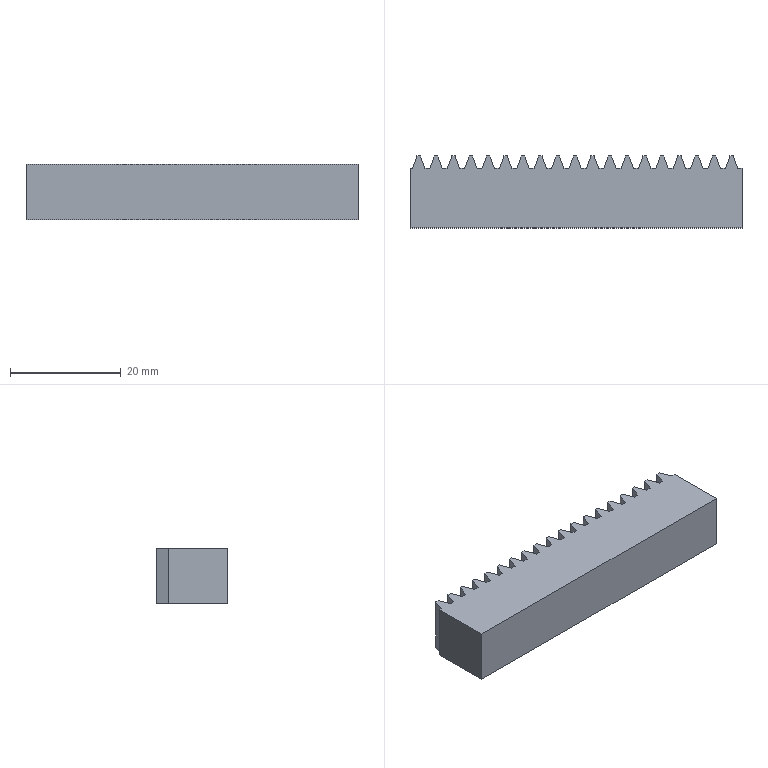Part | STEP file | rack spur rectangular_iso_ISO - Rack-spur - rectangular 1M 20PA 10FW 12PH 60L---SAll | 1 solid | 82 faces | box 60 x 13 x 10 mm | volume 7063 mm3 | plane 82